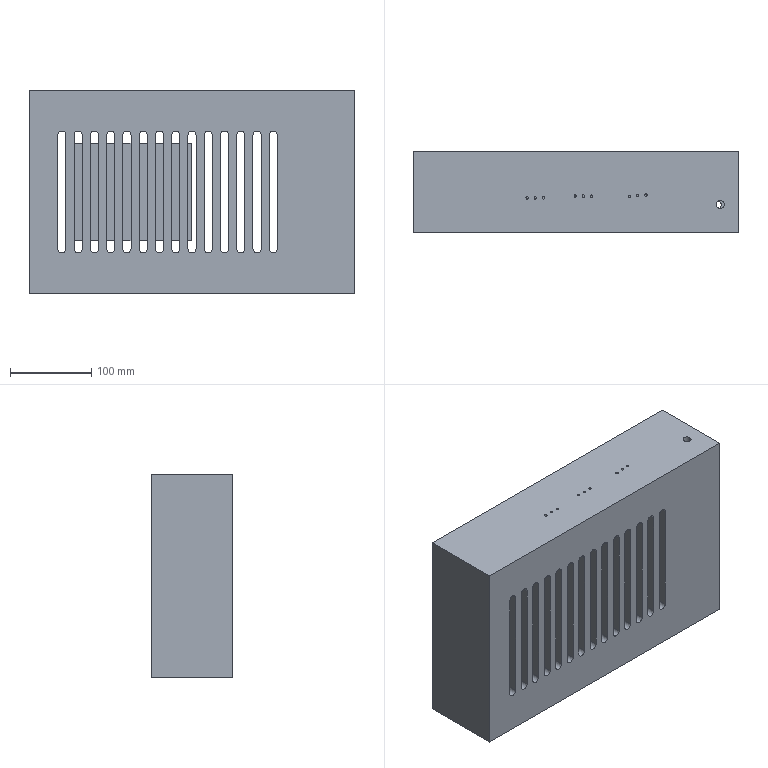Part | SolidWorks | features ICE 7, Extrusion 1, Shell 1 | 1 solid | 136 faces | box 400 x 100 x 250 mm | volume 2452161 mm3 | cylinder 82 | plane 54 | commonest cylinder face diameters 10 x46 3 x36